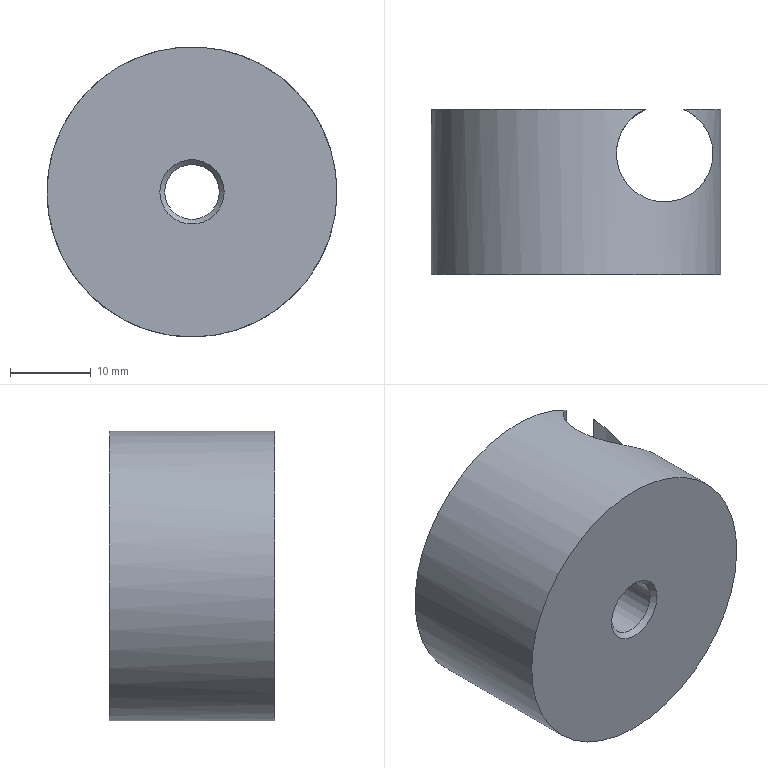Part | STEP file | 冲床-300配套压波_id462_x_t | 1 solid | 8 faces | box 36 x 20.5 x 36 mm | volume 17065 mm3 | cylinder 3 | plane 3 | cone 2 | commonest cylinder face diameters 6.8 x1 12 x1 36 x1
STEP:
#1=CARTESIAN_POINT('',(1108.,-134.,-103.));
#2=VERTEX_POINT('',#1);
#3=CARTESIAN_POINT('',(1126.,-134.,-103.));
#4=DIRECTION('',(0.,1.,0.));
#5=DIRECTION('',(-1.,0.,0.));
#6=AXIS2_PLACEMENT_3D('',#3,#4,#5);
#7=CIRCLE('',#6,18.);
#8=EDGE_CURVE('',#2,#2,#7,.T.);
#9=ORIENTED_EDGE('',*,*,#8,.T.);
#10=EDGE_LOOP('',(#9));
#11=FACE_BOUND('',#10,.T.);
#12=CARTESIAN_POINT('',(1134.602,-113.5,-118.812));
#13=VERTEX_POINT('',#12);
#14=CARTESIAN_POINT('',(1134.602,-113.5,-87.188));
#15=VERTEX_POINT('',#14);
#16=CARTESIAN_POINT('',(1126.,-113.5,-103.));
#17=DIRECTION('',(0.,1.,0.));
#18=DIRECTION('',(0.,0.,1.));
#19=AXIS2_PLACEMENT_3D('',#16,#17,#18);
#20=CIRCLE('',#19,18.);
#21=EDGE_CURVE('',#13,#15,#20,.T.);
#22=ORIENTED_EDGE('',*,*,#21,.F.);
#23=CARTESIAN_POINT('',(1139.398,-113.5,-115.021));
#24=VERTEX_POINT('',#23);
#25=CARTESIAN_POINT('',(1134.602,-113.5,-118.812));
#26=CARTESIAN_POINT('',(1133.24,-114.094,-119.553));
#27=CARTESIAN_POINT('',(1132.004,-115.299,-119.98));
#28=CARTESIAN_POINT('',(1130.819,-118.333,-120.354));
#29=CARTESIAN_POINT('',(1130.881,-120.122,-120.342));
#30=CARTESIAN_POINT('',(1132.307,-123.083,-119.876));
#31=CARTESIAN_POINT('',(1133.626,-124.167,-119.38));
#32=CARTESIAN_POINT('',(1136.345,-125.136,-117.814));
#33=CARTESIAN_POINT('',(1137.718,-125.071,-116.756));
#34=CARTESIAN_POINT('',(1139.952,-124.354,-114.484));
#35=CARTESIAN_POINT('',(1140.872,-123.711,-113.238));
#36=CARTESIAN_POINT('',(1141.928,-122.466,-111.415));
#37=CARTESIAN_POINT('',(1142.234,-121.995,-110.8));
#38=CARTESIAN_POINT('',(1142.724,-120.896,-109.684));
#39=CARTESIAN_POINT('',(1142.926,-120.234,-109.126));
#40=CARTESIAN_POINT('',(1143.042,-118.631,-108.796));
#41=CARTESIAN_POINT('',(1142.914,-117.796,-109.18));
#42=CARTESIAN_POINT('',(1142.514,-116.546,-110.181));
#43=CARTESIAN_POINT('',(1142.245,-116.034,-110.782));
#44=CARTESIAN_POINT('',(1141.293,-114.663,-112.59));
#45=CARTESIAN_POINT('',(1140.458,-113.962,-113.839));
#46=CARTESIAN_POINT('',(1139.398,-113.5,-115.021));
#47=B_SPLINE_CURVE_WITH_KNOTS('',3,(#25,#26,#27,#28,#29,#30,#31,#32,#33,#34,#35,#36,#37,#38,#39,#40,#41,#42,#43,#44,#45,#46),.UNSPECIFIED.,.F.,.F.,(4,2,2,2,2,2,2,2,2,2,4),(0.,0.125,0.25,0.375,0.5,0.625,0.6875,0.75,0.8125,0.875,1.),.UNSPECIFIED.);
#48=EDGE_CURVE('',#13,#24,#47,.T.);
#49=ORIENTED_EDGE('',*,*,#48,.T.);
#50=CARTESIAN_POINT('',(1139.398,-113.5,-90.979));
#51=VERTEX_POINT('',#50);
#52=CARTESIAN_POINT('',(1126.,-113.5,-103.));
#53=DIRECTION('',(0.,1.,0.));
#54=DIRECTION('',(1.,0.,0.));
#55=AXIS2_PLACEMENT_3D('',#52,#53,#54);
#56=CIRCLE('',#55,18.);
#57=EDGE_CURVE('',#51,#24,#56,.T.);
#58=ORIENTED_EDGE('',*,*,#57,.F.);
#59=CARTESIAN_POINT('',(1139.398,-113.5,-90.979));
#60=CARTESIAN_POINT('',(1140.459,-113.963,-92.162));
#61=CARTESIAN_POINT('',(1141.29,-114.659,-93.404));
#62=CARTESIAN_POINT('',(1142.247,-116.037,-95.222));
#63=CARTESIAN_POINT('',(1142.516,-116.55,-95.822));
#64=CARTESIAN_POINT('',(1142.914,-117.795,-96.819));
#65=CARTESIAN_POINT('',(1143.043,-118.626,-97.205));
#66=CARTESIAN_POINT('',(1142.926,-120.24,-96.873));
#67=CARTESIAN_POINT('',(1142.724,-120.896,-96.316));
#68=CARTESIAN_POINT('',(1142.234,-121.995,-95.201));
#69=CARTESIAN_POINT('',(1141.928,-122.466,-94.586));
#70=CARTESIAN_POINT('',(1140.87,-123.713,-92.76));
#71=CARTESIAN_POINT('',(1139.953,-124.354,-91.517));
#72=CARTESIAN_POINT('',(1137.718,-125.071,-89.244));
#73=CARTESIAN_POINT('',(1136.353,-125.137,-88.191));
#74=CARTESIAN_POINT('',(1133.63,-124.17,-86.621));
#75=CARTESIAN_POINT('',(1132.309,-123.077,-86.125));
#76=CARTESIAN_POINT('',(1130.893,-120.157,-85.662));
#77=CARTESIAN_POINT('',(1130.812,-118.36,-85.644));
#78=CARTESIAN_POINT('',(1132.004,-115.293,-86.019));
#79=CARTESIAN_POINT('',(1133.238,-114.095,-86.446));
#80=CARTESIAN_POINT('',(1134.602,-113.5,-87.188));
#81=B_SPLINE_CURVE_WITH_KNOTS('',3,(#59,#60,#61,#62,#63,#64,#65,#66,#67,#68,#69,#70,#71,#72,#73,#74,#75,#76,#77,#78,#79,#80),.UNSPECIFIED.,.F.,.F.,(4,2,2,2,2,2,2,2,2,2,4),(0.,0.125,0.1875,0.25,0.3125,0.375,0.5,0.625,0.75,0.875,1.),.UNSPECIFIED.);
#82=EDGE_CURVE('',#51,#15,#81,.T.);
#83=ORIENTED_EDGE('',*,*,#82,.T.);
#84=EDGE_LOOP('',(#22,#49,#58,#83));
#85=FACE_BOUND('',#84,.T.);
#86=CARTESIAN_POINT('',(1126.,-134.,-103.));
#87=DIRECTION('',(0.,1.,0.));
#88=DIRECTION('',(0.,0.,1.));
#89=AXIS2_PLACEMENT_3D('',#86,#87,#88);
#90=CYLINDRICAL_SURFACE('',#89,18.);
#91=ADVANCED_FACE('',(#11,#85),#90,.T.);
#92=CARTESIAN_POINT('',(1130.,-113.5,-103.));
#93=VERTEX_POINT('',#92);
#94=CARTESIAN_POINT('',(1126.,-113.5,-103.));
#95=DIRECTION('',(0.,-1.,0.));
#96=DIRECTION('',(1.,0.,0.));
#97=AXIS2_PLACEMENT_3D('',#94,#95,#96);
#98=CIRCLE('',#97,4.);
#99=EDGE_CURVE('',#93,#93,#98,.T.);
#100=ORIENTED_EDGE('',*,*,#99,.T.);
#101=EDGE_LOOP('',(#100));
#102=FACE_BOUND('',#101,.T.);
#103=ORIENTED_EDGE('',*,*,#21,.T.);
#104=CARTESIAN_POINT('',(1134.602,-113.5,-57.));
#105=DIRECTION('',(0.,0.,-1.));
#106=VECTOR('',#105,1.);
#107=LINE('',#104,#106);
#108=EDGE_CURVE('',#15,#13,#107,.T.);
#109=ORIENTED_EDGE('',*,*,#108,.T.);
#110=EDGE_LOOP('',(#103,#109));
#111=FACE_BOUND('',#110,.T.);
#112=CARTESIAN_POINT('',(1126.,-113.5,-103.));
#113=DIRECTION('',(0.,1.,0.));
#114=DIRECTION('',(0.,0.,1.));
#115=AXIS2_PLACEMENT_3D('',#112,#113,#114);
#116=PLANE('',#115);
#117=ADVANCED_FACE('',(#102,#111),#116,.T.);
#118=ORIENTED_EDGE('',*,*,#57,.T.);
#119=CARTESIAN_POINT('',(1139.398,-113.5,-57.));
#120=DIRECTION('',(0.,0.,1.));
#121=VECTOR('',#120,1.);
#122=LINE('',#119,#121);
#123=EDGE_CURVE('',#24,#51,#122,.T.);
#124=ORIENTED_EDGE('',*,*,#123,.T.);
#125=EDGE_LOOP('',(#118,#124));
#126=FACE_OUTER_BOUND('',#125,.T.);
#127=CARTESIAN_POINT('',(1127.,-113.5,-103.));
#128=DIRECTION('',(0.,1.,0.));
#129=DIRECTION('',(0.,0.,1.));
#130=AXIS2_PLACEMENT_3D('',#127,#128,#129);
#131=PLANE('',#130);
#132=ADVANCED_FACE('',(#126),#131,.T.);
#133=CARTESIAN_POINT('',(1130.,-134.,-103.));
#134=VERTEX_POINT('',#133);
#135=CARTESIAN_POINT('',(1126.,-134.,-103.));
#136=DIRECTION('',(0.,1.,0.));
#137=DIRECTION('',(1.,0.,0.));
#138=AXIS2_PLACEMENT_3D('',#135,#136,#137);
#139=CIRCLE('',#138,4.);
#140=EDGE_CURVE('',#134,#134,#139,.T.);
#141=ORIENTED_EDGE('',*,*,#140,.T.);
#142=EDGE_LOOP('',(#141));
#143=FACE_BOUND('',#142,.T.);
#144=ORIENTED_EDGE('',*,*,#8,.F.);
#145=EDGE_LOOP('',(#144));
#146=FACE_BOUND('',#145,.T.);
#147=CARTESIAN_POINT('',(1126.,-134.,-103.));
#148=DIRECTION('',(0.,1.,0.));
#149=DIRECTION('',(0.,0.,1.));
#150=AXIS2_PLACEMENT_3D('',#147,#148,#149);
#151=PLANE('',#150);
#152=ADVANCED_FACE('',(#143,#146),#151,.F.);
#153=ORIENTED_EDGE('',*,*,#48,.F.);
#154=ORIENTED_EDGE('',*,*,#108,.F.);
#155=ORIENTED_EDGE('',*,*,#82,.F.);
#156=ORIENTED_EDGE('',*,*,#123,.F.);
#157=EDGE_LOOP('',(#153,#154,#155,#156));
#158=FACE_OUTER_BOUND('',#157,.T.);
#159=CARTESIAN_POINT('',(1137.,-119.,-57.));
#160=DIRECTION('',(0.,0.,-1.));
#161=DIRECTION('',(1.,0.,0.));
#162=AXIS2_PLACEMENT_3D('',#159,#160,#161);
#163=CYLINDRICAL_SURFACE('',#162,6.);
#164=ADVANCED_FACE('',(#158),#163,.F.);
#165=CARTESIAN_POINT('',(1129.4,-133.4,-103.));
#166=VERTEX_POINT('',#165);
#167=CARTESIAN_POINT('',(1126.,-133.4,-103.));
#168=DIRECTION('',(0.,-1.,0.));
#169=DIRECTION('',(1.,0.,0.));
#170=AXIS2_PLACEMENT_3D('',#167,#168,#169);
#171=CIRCLE('',#170,3.4);
#172=EDGE_CURVE('',#166,#166,#171,.T.);
#173=ORIENTED_EDGE('',*,*,#172,.T.);
#174=EDGE_LOOP('',(#173));
#175=FACE_BOUND('',#174,.T.);
#176=CARTESIAN_POINT('',(1129.4,-114.1,-103.));
#177=VERTEX_POINT('',#176);
#178=CARTESIAN_POINT('',(1126.,-114.1,-103.));
#179=DIRECTION('',(0.,1.,0.));
#180=DIRECTION('',(1.,0.,0.));
#181=AXIS2_PLACEMENT_3D('',#178,#179,#180);
#182=CIRCLE('',#181,3.4);
#183=EDGE_CURVE('',#177,#177,#182,.T.);
#184=ORIENTED_EDGE('',*,*,#183,.T.);
#185=EDGE_LOOP('',(#184));
#186=FACE_BOUND('',#185,.T.);
#187=CARTESIAN_POINT('',(1126.,-67.,-103.));
#188=DIRECTION('',(0.,-1.,0.));
#189=DIRECTION('',(-1.,0.,0.));
#190=AXIS2_PLACEMENT_3D('',#187,#188,#189);
#191=CYLINDRICAL_SURFACE('',#190,3.4);
#192=ADVANCED_FACE('',(#175,#186),#191,.F.);
#193=ORIENTED_EDGE('',*,*,#140,.F.);
#194=EDGE_LOOP('',(#193));
#195=FACE_BOUND('',#194,.T.);
#196=ORIENTED_EDGE('',*,*,#172,.F.);
#197=EDGE_LOOP('',(#196));
#198=FACE_BOUND('',#197,.T.);
#199=CARTESIAN_POINT('',(1126.,-133.4,-103.));
#200=DIRECTION('',(0.,-1.,0.));
#201=DIRECTION('',(-1.,0.,0.));
#202=AXIS2_PLACEMENT_3D('',#199,#200,#201);
#203=CONICAL_SURFACE('',#202,3.4,45.);
#204=ADVANCED_FACE('',(#195,#198),#203,.F.);
#205=ORIENTED_EDGE('',*,*,#183,.F.);
#206=EDGE_LOOP('',(#205));
#207=FACE_BOUND('',#206,.T.);
#208=ORIENTED_EDGE('',*,*,#99,.F.);
#209=EDGE_LOOP('',(#208));
#210=FACE_BOUND('',#209,.T.);
#211=CARTESIAN_POINT('',(1126.,-113.5,-103.));
#212=DIRECTION('',(0.,1.,0.));
#213=DIRECTION('',(1.,0.,0.));
#214=AXIS2_PLACEMENT_3D('',#211,#212,#213);
#215=CONICAL_SURFACE('',#214,4.,45.);
#216=ADVANCED_FACE('',(#207,#210),#215,.F.);
#217=CLOSED_SHELL('',(#91,#117,#132,#152,#164,#192,#204,#216));
#218=MANIFOLD_SOLID_BREP('',#217);
#219=(LENGTH_UNIT()NAMED_UNIT(*)SI_UNIT(.MILLI.,.METRE.));
#220=UNCERTAINTY_MEASURE_WITH_UNIT(LENGTH_MEASURE(0.0508),#219,'','');
#221=(NAMED_UNIT(*)PLANE_ANGLE_UNIT()SI_UNIT($,.RADIAN.));
#222=PLANE_ANGLE_MEASURE_WITH_UNIT(PLANE_ANGLE_MEASURE(0.01745),#221);
#223=DIMENSIONAL_EXPONENTS(0.,0.,0.,0.,0.,0.,0.);
#224=(CONVERSION_BASED_UNIT('DEGREE',#222)NAMED_UNIT(#223)PLANE_ANGLE_UNIT());
#225=(NAMED_UNIT(*)SI_UNIT($,.STERADIAN.)SOLID_ANGLE_UNIT());
#226=(GEOMETRIC_REPRESENTATION_CONTEXT(3)GLOBAL_UNCERTAINTY_ASSIGNED_CONTEXT((#220))GLOBAL_UNIT_ASSIGNED_CONTEXT((#219,#224,#225))REPRESENTATION_CONTEXT('',''));
#227=ADVANCED_BREP_SHAPE_REPRESENTATION('',(#218),#226);